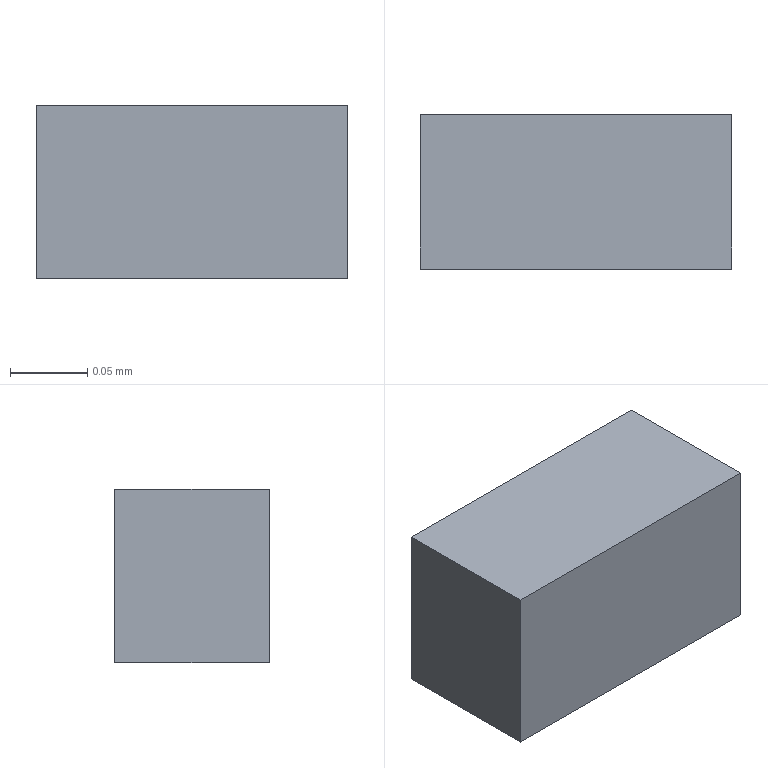Part | Creo | 1 solid | 6 faces | box 0.2016 x 0.1 x 0.1125 mm | volume 0.002268 mm3 | plane 6
STEP:
#1=CARTESIAN_POINT('',(0.,0.,0.));
#2=DIRECTION('',(0.,0.,1.));
#3=DIRECTION('',(1.,0.,0.));
#4=AXIS2_PLACEMENT_3D('',#1,#2,#3);
#5=CARTESIAN_POINT('',(-0.1008,-0.05,0.));
#6=VERTEX_POINT('',#5);
#7=CARTESIAN_POINT('',(0.1008,-0.05,0.));
#8=VERTEX_POINT('',#7);
#9=CARTESIAN_POINT('',(-0.1008,-0.05,0.));
#10=DIRECTION('',(1.,0.,0.));
#11=VECTOR('',#10,0.2016);
#12=LINE('',#9,#11);
#13=EDGE_CURVE('',#6,#8,#12,.T.);
#14=ORIENTED_EDGE('',*,*,#13,.T.);
#15=CARTESIAN_POINT('',(0.1008,0.05,0.));
#16=VERTEX_POINT('',#15);
#17=CARTESIAN_POINT('',(0.1008,-0.05,0.));
#18=DIRECTION('',(0.,1.,0.));
#19=VECTOR('',#18,0.1);
#20=LINE('',#17,#19);
#21=EDGE_CURVE('',#8,#16,#20,.T.);
#22=ORIENTED_EDGE('',*,*,#21,.T.);
#23=CARTESIAN_POINT('',(-0.1008,0.05,0.));
#24=VERTEX_POINT('',#23);
#25=CARTESIAN_POINT('',(0.1008,0.05,0.));
#26=DIRECTION('',(-1.,0.,0.));
#27=VECTOR('',#26,0.2016);
#28=LINE('',#25,#27);
#29=EDGE_CURVE('',#16,#24,#28,.T.);
#30=ORIENTED_EDGE('',*,*,#29,.T.);
#31=CARTESIAN_POINT('',(-0.1008,0.05,0.));
#32=DIRECTION('',(0.,-1.,0.));
#33=VECTOR('',#32,0.1);
#34=LINE('',#31,#33);
#35=EDGE_CURVE('',#24,#6,#34,.T.);
#36=ORIENTED_EDGE('',*,*,#35,.T.);
#37=EDGE_LOOP('',(#14,#22,#30,#36));
#38=FACE_OUTER_BOUND('',#37,.F.);
#39=CARTESIAN_POINT('',(0.,0.,0.));
#40=DIRECTION('',(0.,0.,1.));
#41=DIRECTION('',(1.,0.,0.));
#42=AXIS2_PLACEMENT_3D('',#39,#40,#41);
#43=PLANE('',#42);
#44=ADVANCED_FACE('',(#38),#43,.F.);
#45=ORIENTED_EDGE('',*,*,#13,.F.);
#46=CARTESIAN_POINT('',(-0.1008,-0.05,0.1125));
#47=VERTEX_POINT('',#46);
#48=CARTESIAN_POINT('',(-0.1008,-0.05,0.));
#49=DIRECTION('',(0.,0.,1.));
#50=VECTOR('',#49,0.1125);
#51=LINE('',#48,#50);
#52=EDGE_CURVE('',#6,#47,#51,.T.);
#53=ORIENTED_EDGE('',*,*,#52,.T.);
#54=CARTESIAN_POINT('',(0.1008,-0.05,0.1125));
#55=VERTEX_POINT('',#54);
#56=CARTESIAN_POINT('',(-0.1008,-0.05,0.1125));
#57=DIRECTION('',(1.,0.,0.));
#58=VECTOR('',#57,0.2016);
#59=LINE('',#56,#58);
#60=EDGE_CURVE('',#47,#55,#59,.T.);
#61=ORIENTED_EDGE('',*,*,#60,.T.);
#62=CARTESIAN_POINT('',(0.1008,-0.05,0.));
#63=DIRECTION('',(0.,0.,1.));
#64=VECTOR('',#63,0.1125);
#65=LINE('',#62,#64);
#66=EDGE_CURVE('',#8,#55,#65,.T.);
#67=ORIENTED_EDGE('',*,*,#66,.F.);
#68=EDGE_LOOP('',(#45,#53,#61,#67));
#69=FACE_OUTER_BOUND('',#68,.F.);
#70=CARTESIAN_POINT('',(-0.1008,-0.05,0.));
#71=DIRECTION('',(0.,-1.,0.));
#72=DIRECTION('',(1.,0.,0.));
#73=AXIS2_PLACEMENT_3D('',#70,#71,#72);
#74=PLANE('',#73);
#75=ADVANCED_FACE('',(#69),#74,.T.);
#76=ORIENTED_EDGE('',*,*,#35,.F.);
#77=CARTESIAN_POINT('',(-0.1008,0.05,0.1125));
#78=VERTEX_POINT('',#77);
#79=CARTESIAN_POINT('',(-0.1008,0.05,0.));
#80=DIRECTION('',(0.,0.,1.));
#81=VECTOR('',#80,0.1125);
#82=LINE('',#79,#81);
#83=EDGE_CURVE('',#24,#78,#82,.T.);
#84=ORIENTED_EDGE('',*,*,#83,.T.);
#85=CARTESIAN_POINT('',(-0.1008,0.05,0.1125));
#86=DIRECTION('',(0.,-1.,0.));
#87=VECTOR('',#86,0.1);
#88=LINE('',#85,#87);
#89=EDGE_CURVE('',#78,#47,#88,.T.);
#90=ORIENTED_EDGE('',*,*,#89,.T.);
#91=ORIENTED_EDGE('',*,*,#52,.F.);
#92=EDGE_LOOP('',(#76,#84,#90,#91));
#93=FACE_OUTER_BOUND('',#92,.F.);
#94=CARTESIAN_POINT('',(-0.1008,0.05,0.));
#95=DIRECTION('',(-1.,0.,0.));
#96=DIRECTION('',(0.,-1.,0.));
#97=AXIS2_PLACEMENT_3D('',#94,#95,#96);
#98=PLANE('',#97);
#99=ADVANCED_FACE('',(#93),#98,.T.);
#100=ORIENTED_EDGE('',*,*,#29,.F.);
#101=CARTESIAN_POINT('',(0.1008,0.05,0.1125));
#102=VERTEX_POINT('',#101);
#103=CARTESIAN_POINT('',(0.1008,0.05,0.));
#104=DIRECTION('',(0.,0.,1.));
#105=VECTOR('',#104,0.1125);
#106=LINE('',#103,#105);
#107=EDGE_CURVE('',#16,#102,#106,.T.);
#108=ORIENTED_EDGE('',*,*,#107,.T.);
#109=CARTESIAN_POINT('',(0.1008,0.05,0.1125));
#110=DIRECTION('',(-1.,0.,0.));
#111=VECTOR('',#110,0.2016);
#112=LINE('',#109,#111);
#113=EDGE_CURVE('',#102,#78,#112,.T.);
#114=ORIENTED_EDGE('',*,*,#113,.T.);
#115=ORIENTED_EDGE('',*,*,#83,.F.);
#116=EDGE_LOOP('',(#100,#108,#114,#115));
#117=FACE_OUTER_BOUND('',#116,.F.);
#118=CARTESIAN_POINT('',(0.1008,0.05,0.));
#119=DIRECTION('',(0.,1.,0.));
#120=DIRECTION('',(-1.,0.,0.));
#121=AXIS2_PLACEMENT_3D('',#118,#119,#120);
#122=PLANE('',#121);
#123=ADVANCED_FACE('',(#117),#122,.T.);
#124=ORIENTED_EDGE('',*,*,#21,.F.);
#125=ORIENTED_EDGE('',*,*,#66,.T.);
#126=CARTESIAN_POINT('',(0.1008,-0.05,0.1125));
#127=DIRECTION('',(0.,1.,0.));
#128=VECTOR('',#127,0.1);
#129=LINE('',#126,#128);
#130=EDGE_CURVE('',#55,#102,#129,.T.);
#131=ORIENTED_EDGE('',*,*,#130,.T.);
#132=ORIENTED_EDGE('',*,*,#107,.F.);
#133=EDGE_LOOP('',(#124,#125,#131,#132));
#134=FACE_OUTER_BOUND('',#133,.F.);
#135=CARTESIAN_POINT('',(0.1008,-0.05,0.));
#136=DIRECTION('',(1.,0.,0.));
#137=DIRECTION('',(0.,1.,0.));
#138=AXIS2_PLACEMENT_3D('',#135,#136,#137);
#139=PLANE('',#138);
#140=ADVANCED_FACE('',(#134),#139,.T.);
#141=ORIENTED_EDGE('',*,*,#60,.F.);
#142=ORIENTED_EDGE('',*,*,#89,.F.);
#143=ORIENTED_EDGE('',*,*,#113,.F.);
#144=ORIENTED_EDGE('',*,*,#130,.F.);
#145=EDGE_LOOP('',(#141,#142,#143,#144));
#146=FACE_OUTER_BOUND('',#145,.F.);
#147=CARTESIAN_POINT('',(0.,0.,0.1125));
#148=DIRECTION('',(0.,0.,1.));
#149=DIRECTION('',(1.,0.,0.));
#150=AXIS2_PLACEMENT_3D('',#147,#148,#149);
#151=PLANE('',#150);
#152=ADVANCED_FACE('',(#146),#151,.T.);
#153=CLOSED_SHELL('',(#44,#75,#99,#123,#140,#152));
#154=MANIFOLD_SOLID_BREP('',#153);
#155=(LENGTH_UNIT()NAMED_UNIT(*)SI_UNIT(.MILLI.,.METRE.));
#156=UNCERTAINTY_MEASURE_WITH_UNIT(LENGTH_MEASURE(0.00002516),#155,'','');
#157=(NAMED_UNIT(*)PLANE_ANGLE_UNIT()SI_UNIT($,.RADIAN.));
#158=PLANE_ANGLE_MEASURE_WITH_UNIT(PLANE_ANGLE_MEASURE(0.01745),#157);
#159=(CONVERSION_BASED_UNIT('DEGREE',#158)NAMED_UNIT(*)PLANE_ANGLE_UNIT());
#160=(NAMED_UNIT(*)SI_UNIT($,.STERADIAN.)SOLID_ANGLE_UNIT());
#161=(GEOMETRIC_REPRESENTATION_CONTEXT(3)GLOBAL_UNCERTAINTY_ASSIGNED_CONTEXT((#156))GLOBAL_UNIT_ASSIGNED_CONTEXT((#155,#159,#160))REPRESENTATION_CONTEXT('',''));
#162=ADVANCED_BREP_SHAPE_REPRESENTATION('',(#4,#154),#161);